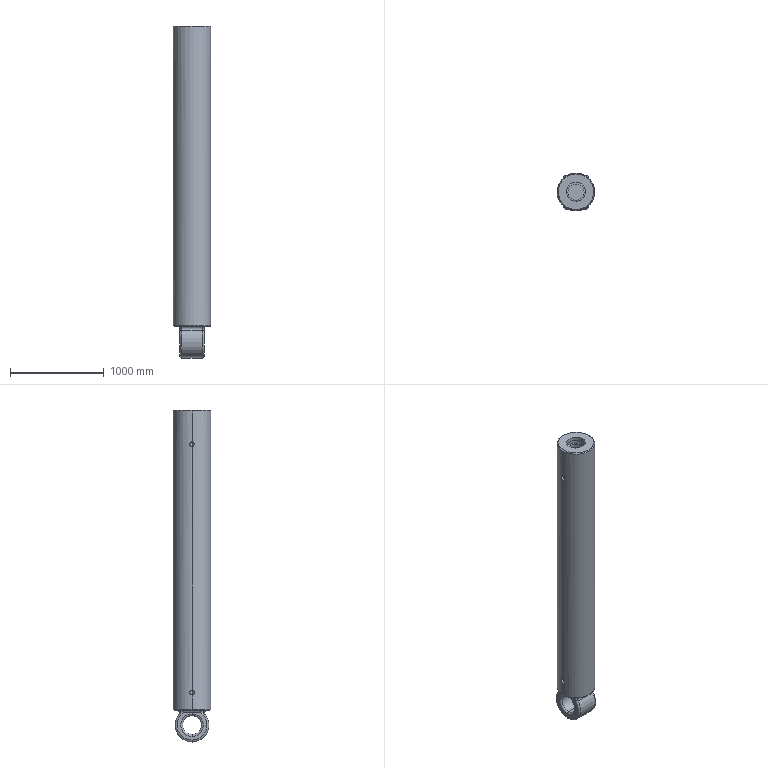Part | SolidWorks | features ICE 10, Fillet 3, RevCut 2, Chamfer 1, Extrusion 1 | 2 solids | 85 faces | box 400 x 400 x 3541 mm | volume 139018402 mm3 | spline 28 | cylinder 26 | torus 15 | plane 14 | cone 2 | commonest cylinder face diameters 201 x6 50 x4 60 x4 171.677 x2 200 x2 230 x2